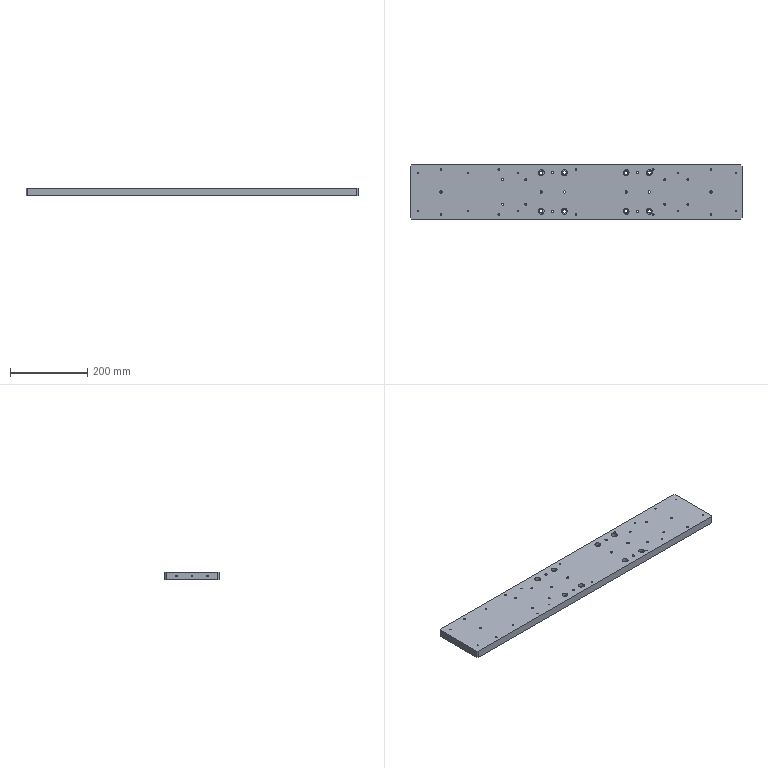CAM job | NX | 3-axis milling, drilling | part box 860 x 140 x 20 mm | stock box 860 x 140 x 20 mm
Tools:
number,name,description,diameter,corner_radius,flute_length,length,flutes
8,D8,平底铣刀-粗,8.0,0.0,30.0,75.0,2
9,D10,平底铣刀-粗,10.0,0.0,35.0,75.0,2
7,D6-J,平底铣刀-精,6.0,0.0,25.0,75.0,2
10,D10-J,平底铣刀-精,10.0,0.0,35.0,75.0,2
2,D6倒角刀,倒角刀,6.0,0.0,3.0,25.0,2
21,M4X0.7,丝锥,3.3,0.0,35.0,50.0,2
22,M5X0.8,丝锥,4.2,0.0,35.0,50.0,2
23,M6X1.0,丝锥,5.0,0.0,35.0,50.0,2
19,D6铰刀,Drilling Tool,6.0,0.0,75.0,100.0,6
1,C6定点钻,倒角刀,6.0,0.0,3.0,3.0,2
13,ZT3.4,钻头,3.4,0.0,35.0,50.0,2
15,ZT5.1,钻头,5.1,0.0,35.0,50.0,2
18,ZT9,钻头,9.0,0.0,35.0,50.0,2
17,ZT5.9,Drilling Tool,5.9,0.0,35.0,50.0,2
20,ZT4.3,Drilling Tool,4.3,0.0,50.0,75.0,4
Operations:
program,operation,operation_type,tool,method,geometry_group,spindle_rpm,surface_speed,feed_per_tooth,feed_cut,feed_plunge,cut_length_mm,path_length_mm,cut_time_min,machine_time_min
B,等高往复层切开粗-中_COPY_COPY,ZLevelMilling,D10,分层开粗-切深K-步距G,W-B,3000.0,94.245,0.3333,2000.0,100.0,2894.048,4296.601,1.447,1.587
B,钻倒角_2,Operation,D6倒角刀,METHOD,W-B,2000.0,0.0,0.025,100.0,0.0,52.0,1496.335,0.52,0.6644
B,钻倒角_3,Operation,D6倒角刀,METHOD,W-B,2000.0,0.0,0.025,100.0,0.0,57.0,1461.299,0.57,0.7104
B,铣倒角_5,PlanarMilling,D6倒角刀,METHOD,W-B,4000.0,75.398,0.0375,300.0,100.0,144.163,1209.83,0.4805,0.5871
B,铣倒角_6,PlanarMilling,D6倒角刀,METHOD,W-B,4000.0,75.398,0.075,600.0,100.0,180.203,1617.449,0.3003,0.4441
B,铣倒角_7,PlanarMilling,D6倒角刀,METHOD,W-B,3000.0,56.549,0.1,600.0,100.0,187.355,1136.483,0.3123,0.4072
B,C0.3封闭铣廓倒角6X45L_COPY_1,PlanarMilling,D6倒角刀,爬面_倒角-切深0-步距G,W-B,4000.0,75.398,0.125,1000.0,100.0,2015.102,2051.602,2.015,2.019
B,等高精光-中_COPY_COPY,ZLevelMilling,D10-J,侧刃精光-切深K-步距G,W-B,3000.0,94.245,0.1333,800.0,100.0,44.032,1307.354,0.055,0.1814
A,等高往复层切开粗-中_COPY,ZLevelMilling,D10,分层开粗-切深K-步距G,W-A,3000.0,94.245,0.3333,2000.0,100.0,2894.048,4536.601,1.447,1.611
A,打点-深0.8,Operation,C6定点钻,NONE,W-A,3000.0,56.0,0.01,60.0,90.0,82.8,2507.853,1.38,1.623
A,通孔-M4螺纹底孔,Operation,ZT3.4,NONE,W-A,1500.0,15.551,0.02,60.0,90.0,270.0,1974.037,4.5,4.67
A,通孔-M5螺纹底孔,Operation,ZT4.3,NONE,W-A,1200.0,15.834,0.0333,80.0,90.0,270.0,1929.033,3.375,3.541
A,通孔-M6螺纹底孔,Operation,ZT5.1,NONE,W-A,800.0,12.566,0.0625,100.0,90.0,216.0,1267.05,2.16,2.265
A,通孔-精孔6.0预钻,Operation,ZT5.9,NONE,W-A,1000.0,18.535,0.04,80.0,90.0,257.032,1612.979,3.213,3.349
A,沉头孔-钻孔0段,Operation,ZT9,NONE,W-A,500.0,14.137,0.12,120.0,90.0,205.631,1118.308,1.714,1.805
A,铣孔开粗D8_1,CylinderMilling,D8,NONE,W-A,4000.0,100.531,0.25,2000.0,100.0,6477.636,7942.436,3.239,3.385
A,铣孔精光D8_1,CylinderMilling,D6-J,精光步距切深关,W-A,4000.0,100.531,0.1,800.0,100.0,749.192,2213.992,0.9365,1.083
A,钻倒角_1,Operation,D6倒角刀,METHOD,W-A,4000.0,75.398,0.01,80.0,0.0,52.0,1556.335,0.65,0.8004
A,铣倒角_1,PlanarMilling,D6倒角刀,METHOD,W-A,4000.0,75.398,0.025,200.0,100.0,180.203,2471.614,0.901,1.13
A,铣倒角_2,PlanarMilling,D6倒角刀,METHOD,W-A,4000.0,75.398,0.0375,300.0,100.0,159.505,1697.25,0.5317,0.6855
A,铣倒角_3,PlanarMilling,D6倒角刀,METHOD,W-A,4000.0,75.398,0.05,400.0,100.0,209.637,2232.939,0.5241,0.7264
A,铣倒角_4,PlanarMilling,D6倒角刀,NONE,W-A,4000.0,75.398,0.1,800.0,100.0,447.672,1812.197,0.5596,0.696
A,C0.3封闭铣廓倒角6X45L_COPY,PlanarMilling,D6倒角刀,爬面_倒角-切深0-步距G,W-A,4000.0,75.398,0.125,1000.0,100.0,2012.34,2108.54,2.012,2.022
A,铰孔,Operation,D6铰刀,METHOD,W-A,500.0,9.425,0.0167,50.0,0.0,220.0,1538.916,4.4,4.532
A,通孔-攻牙M4,Operation,M4X0.7,METHOD,W-A,500.0,5.184,0.0007,0.7,90.0,245.0,1924.037,350.0,350.168
A,通孔-攻牙M5,Operation,M5X0.8,METHOD,W-A,500.0,6.597,0.0008,0.8,90.0,245.0,1879.033,306.25,306.413
A,通孔-攻牙M6,Operation,M6X1.0,METHOD,W-A,400.0,6.283,0.0013,1.0,90.0,196.0,1227.05,196.0,196.103
A,等高精光-中_COPY,ZLevelMilling,D10-J,侧刃精光-切深K-步距G,W-A,3000.0,94.245,0.1333,800.0,100.0,44.032,1338.138,0.055,0.1845